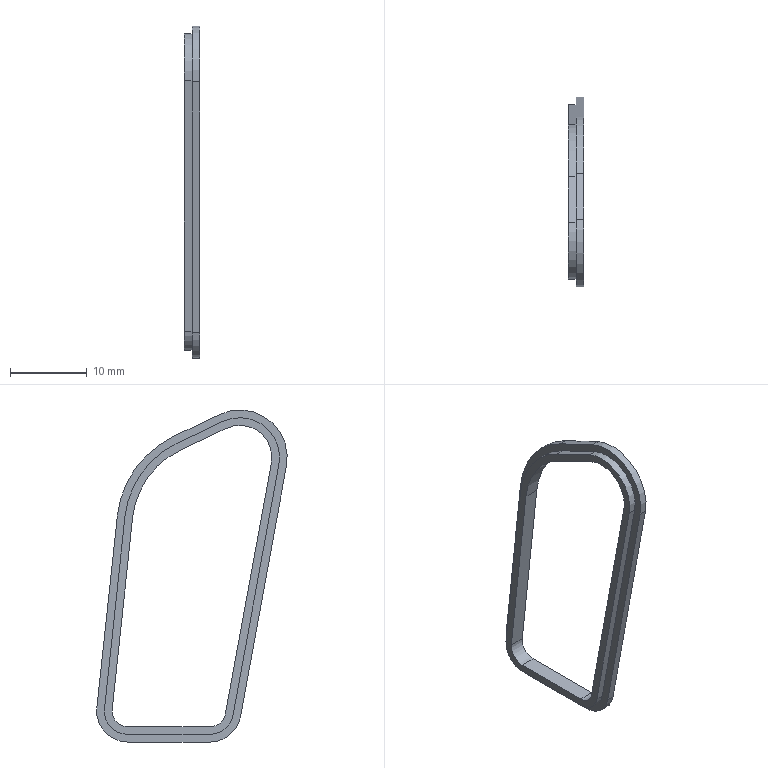Part | STEP file | 1-31.5 | 1 solid | 27 faces | box 2 x 24.769 x 43.162 mm | volume 321.973 mm3 | plane 15 | cylinder 12 | commonest cylinder face diameters 4 x2 6 x2 8 x2 8.325 x1 10.325 x1 12.325 x1